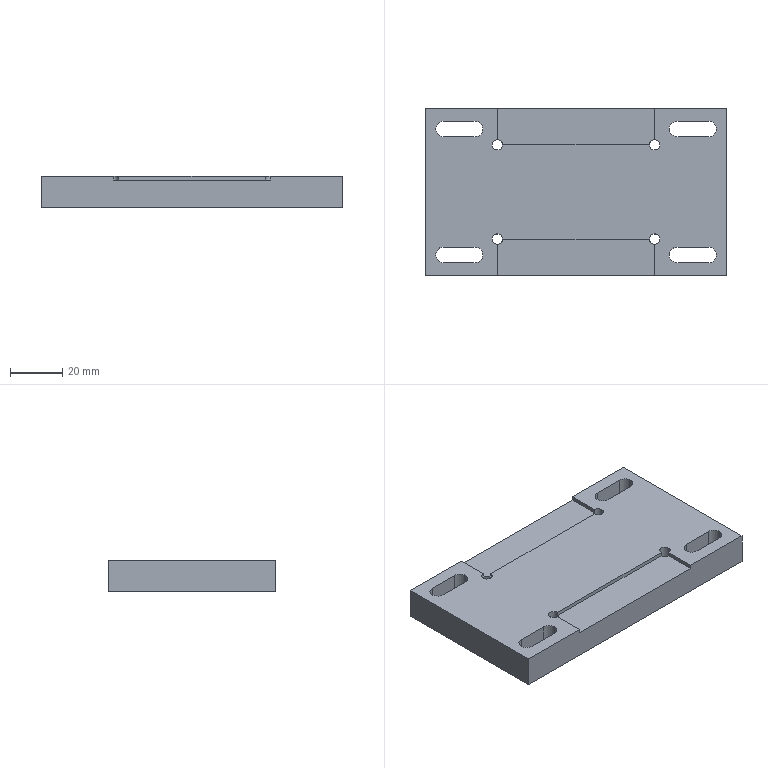Part | SolidWorks | features ICE 3, 3DProfileFeature 1, Extrusion 1, HoleWzd 1, MirrorPattern 1 | 1 solid | 46 faces | box 115 x 64 x 12 mm | volume 80039 mm3 | cylinder 22 | plane 22 | cone 2 | commonest cylinder face diameters 6 x12 4 x8 5 x2
STEP:
#1=CARTESIAN_POINT('',(39.5,0.,2.5));
#2=VERTEX_POINT('',#1);
#3=CARTESIAN_POINT('',(39.5,0.,-2.5));
#4=VERTEX_POINT('',#3);
#5=CARTESIAN_POINT('',(39.5,0.,0.));
#6=DIRECTION('',(1.,0.,0.));
#7=DIRECTION('',(0.,0.,-1.));
#8=AXIS2_PLACEMENT_3D('',#5,#6,#7);
#9=CIRCLE('',#8,2.5);
#10=EDGE_CURVE('',#2,#4,#9,.T.);
#11=ORIENTED_EDGE('',*,*,#10,.F.);
#12=CARTESIAN_POINT('',(57.5,0.,2.5));
#13=VERTEX_POINT('',#12);
#14=CARTESIAN_POINT('',(57.5,0.,2.5));
#15=DIRECTION('',(1.,0.,0.));
#16=VECTOR('',#15,1000.);
#17=LINE('',#14,#16);
#18=EDGE_CURVE('',#2,#13,#17,.T.);
#19=ORIENTED_EDGE('',*,*,#18,.T.);
#20=CARTESIAN_POINT('',(57.5,0.,-2.5));
#21=VERTEX_POINT('',#20);
#22=CARTESIAN_POINT('',(57.5,0.,0.));
#23=DIRECTION('',(1.,0.,0.));
#24=DIRECTION('',(0.,0.,-1.));
#25=AXIS2_PLACEMENT_3D('',#22,#23,#24);
#26=CIRCLE('',#25,2.5);
#27=EDGE_CURVE('',#13,#21,#26,.T.);
#28=ORIENTED_EDGE('',*,*,#27,.T.);
#29=CARTESIAN_POINT('',(57.5,0.,-2.5));
#30=DIRECTION('',(1.,0.,0.));
#31=VECTOR('',#30,1000.);
#32=LINE('',#29,#31);
#33=EDGE_CURVE('',#4,#21,#32,.T.);
#34=ORIENTED_EDGE('',*,*,#33,.F.);
#35=EDGE_LOOP('',(#11,#19,#28,#34));
#36=FACE_OUTER_BOUND('',#35,.T.);
#37=CARTESIAN_POINT('',(57.5,0.,0.));
#38=DIRECTION('',(1.,0.,0.));
#39=DIRECTION('',(0.,0.,-1.));
#40=AXIS2_PLACEMENT_3D('',#37,#38,#39);
#41=CYLINDRICAL_SURFACE('',#40,2.5);
#42=ADVANCED_FACE('',(#36),#41,.F.);
#43=CARTESIAN_POINT('',(37.998,0.,0.));
#44=VERTEX_POINT('',#43);
#45=CARTESIAN_POINT('',(39.5,0.,-2.5));
#46=DIRECTION('',(0.515,0.,-0.8572));
#47=VECTOR('',#46,1000.);
#48=LINE('',#45,#47);
#49=EDGE_CURVE('',#44,#4,#48,.T.);
#50=ORIENTED_EDGE('',*,*,#49,.F.);
#51=CARTESIAN_POINT('',(39.5,0.,2.5));
#52=DIRECTION('',(0.515,0.,0.8572));
#53=VECTOR('',#52,1000.);
#54=LINE('',#51,#53);
#55=EDGE_CURVE('',#44,#2,#54,.T.);
#56=ORIENTED_EDGE('',*,*,#55,.T.);
#57=ORIENTED_EDGE('',*,*,#10,.T.);
#58=EDGE_LOOP('',(#50,#56,#57));
#59=FACE_OUTER_BOUND('',#58,.T.);
#60=CARTESIAN_POINT('',(39.5,0.,0.));
#61=DIRECTION('',(1.,0.,0.));
#62=DIRECTION('',(0.,0.,-1.));
#63=AXIS2_PLACEMENT_3D('',#60,#61,#62);
#64=CONICAL_SURFACE('',#63,2.5,1.03);
#65=ADVANCED_FACE('',(#59),#64,.F.);
#66=CARTESIAN_POINT('',(53.5,24.,-6.));
#67=VERTEX_POINT('',#66);
#68=CARTESIAN_POINT('',(50.5,27.,-6.));
#69=VERTEX_POINT('',#68);
#70=CARTESIAN_POINT('',(50.5,24.,-6.));
#71=DIRECTION('',(0.,0.,1.));
#72=DIRECTION('',(-1.,0.,0.));
#73=AXIS2_PLACEMENT_3D('',#70,#71,#72);
#74=CIRCLE('',#73,3.);
#75=EDGE_CURVE('',#67,#69,#74,.T.);
#76=ORIENTED_EDGE('',*,*,#75,.F.);
#77=CARTESIAN_POINT('',(53.5,24.,6.));
#78=VERTEX_POINT('',#77);
#79=CARTESIAN_POINT('',(53.5,24.,-6.001));
#80=DIRECTION('',(0.,0.,1.));
#81=VECTOR('',#80,1000.);
#82=LINE('',#79,#81);
#83=EDGE_CURVE('',#67,#78,#82,.T.);
#84=ORIENTED_EDGE('',*,*,#83,.T.);
#85=CARTESIAN_POINT('',(50.5,27.,6.));
#86=VERTEX_POINT('',#85);
#87=CARTESIAN_POINT('',(50.5,24.,6.));
#88=DIRECTION('',(0.,0.,1.));
#89=DIRECTION('',(-1.,0.,0.));
#90=AXIS2_PLACEMENT_3D('',#87,#88,#89);
#91=CIRCLE('',#90,3.);
#92=EDGE_CURVE('',#78,#86,#91,.T.);
#93=ORIENTED_EDGE('',*,*,#92,.T.);
#94=CARTESIAN_POINT('',(50.5,27.,-6.001));
#95=DIRECTION('',(0.,0.,1.));
#96=VECTOR('',#95,1000.);
#97=LINE('',#94,#96);
#98=EDGE_CURVE('',#69,#86,#97,.T.);
#99=ORIENTED_EDGE('',*,*,#98,.F.);
#100=EDGE_LOOP('',(#76,#84,#93,#99));
#101=FACE_OUTER_BOUND('',#100,.T.);
#102=CARTESIAN_POINT('',(50.5,24.,-6.001));
#103=DIRECTION('',(0.,0.,1.));
#104=DIRECTION('',(1.,0.,0.));
#105=AXIS2_PLACEMENT_3D('',#102,#103,#104);
#106=CYLINDRICAL_SURFACE('',#105,3.);
#107=ADVANCED_FACE('',(#101),#106,.F.);
#108=CARTESIAN_POINT('',(-35.5,-24.,-6.));
#109=VERTEX_POINT('',#108);
#110=CARTESIAN_POINT('',(-38.5,-21.,-6.));
#111=VERTEX_POINT('',#110);
#112=CARTESIAN_POINT('',(-38.5,-24.,-6.));
#113=DIRECTION('',(0.,0.,1.));
#114=DIRECTION('',(-1.,0.,0.));
#115=AXIS2_PLACEMENT_3D('',#112,#113,#114);
#116=CIRCLE('',#115,3.);
#117=EDGE_CURVE('',#109,#111,#116,.T.);
#118=ORIENTED_EDGE('',*,*,#117,.F.);
#119=CARTESIAN_POINT('',(-35.5,-24.,6.));
#120=VERTEX_POINT('',#119);
#121=CARTESIAN_POINT('',(-35.5,-24.,-6.001));
#122=DIRECTION('',(0.,0.,1.));
#123=VECTOR('',#122,1000.);
#124=LINE('',#121,#123);
#125=EDGE_CURVE('',#109,#120,#124,.T.);
#126=ORIENTED_EDGE('',*,*,#125,.T.);
#127=CARTESIAN_POINT('',(-38.5,-21.,6.));
#128=VERTEX_POINT('',#127);
#129=CARTESIAN_POINT('',(-38.5,-24.,6.));
#130=DIRECTION('',(0.,0.,1.));
#131=DIRECTION('',(-1.,0.,0.));
#132=AXIS2_PLACEMENT_3D('',#129,#130,#131);
#133=CIRCLE('',#132,3.);
#134=EDGE_CURVE('',#120,#128,#133,.T.);
#135=ORIENTED_EDGE('',*,*,#134,.T.);
#136=CARTESIAN_POINT('',(-38.5,-21.,-6.001));
#137=DIRECTION('',(0.,0.,1.));
#138=VECTOR('',#137,1000.);
#139=LINE('',#136,#138);
#140=EDGE_CURVE('',#111,#128,#139,.T.);
#141=ORIENTED_EDGE('',*,*,#140,.F.);
#142=EDGE_LOOP('',(#118,#126,#135,#141));
#143=FACE_OUTER_BOUND('',#142,.T.);
#144=CARTESIAN_POINT('',(-38.5,-24.,-6.001));
#145=DIRECTION('',(0.,0.,1.));
#146=DIRECTION('',(1.,0.,0.));
#147=AXIS2_PLACEMENT_3D('',#144,#145,#146);
#148=CYLINDRICAL_SURFACE('',#147,3.);
#149=ADVANCED_FACE('',(#143),#148,.F.);
#150=CARTESIAN_POINT('',(53.5,-24.,-6.));
#151=VERTEX_POINT('',#150);
#152=CARTESIAN_POINT('',(50.5,-21.,-6.));
#153=VERTEX_POINT('',#152);
#154=CARTESIAN_POINT('',(50.5,-24.,-6.));
#155=DIRECTION('',(0.,0.,1.));
#156=DIRECTION('',(-1.,0.,0.));
#157=AXIS2_PLACEMENT_3D('',#154,#155,#156);
#158=CIRCLE('',#157,3.);
#159=EDGE_CURVE('',#151,#153,#158,.T.);
#160=ORIENTED_EDGE('',*,*,#159,.F.);
#161=CARTESIAN_POINT('',(53.5,-24.,6.));
#162=VERTEX_POINT('',#161);
#163=CARTESIAN_POINT('',(53.5,-24.,-6.001));
#164=DIRECTION('',(0.,0.,1.));
#165=VECTOR('',#164,1000.);
#166=LINE('',#163,#165);
#167=EDGE_CURVE('',#151,#162,#166,.T.);
#168=ORIENTED_EDGE('',*,*,#167,.T.);
#169=CARTESIAN_POINT('',(50.5,-21.,6.));
#170=VERTEX_POINT('',#169);
#171=CARTESIAN_POINT('',(50.5,-24.,6.));
#172=DIRECTION('',(0.,0.,1.));
#173=DIRECTION('',(1.,0.,0.));
#174=AXIS2_PLACEMENT_3D('',#171,#172,#173);
#175=CIRCLE('',#174,3.);
#176=EDGE_CURVE('',#162,#170,#175,.T.);
#177=ORIENTED_EDGE('',*,*,#176,.T.);
#178=CARTESIAN_POINT('',(50.5,-21.,-6.001));
#179=DIRECTION('',(0.,0.,1.));
#180=VECTOR('',#179,1000.);
#181=LINE('',#178,#180);
#182=EDGE_CURVE('',#153,#170,#181,.T.);
#183=ORIENTED_EDGE('',*,*,#182,.F.);
#184=EDGE_LOOP('',(#160,#168,#177,#183));
#185=FACE_OUTER_BOUND('',#184,.T.);
#186=CARTESIAN_POINT('',(50.5,-24.,-6.001));
#187=DIRECTION('',(0.,0.,1.));
#188=DIRECTION('',(1.,0.,0.));
#189=AXIS2_PLACEMENT_3D('',#186,#187,#188);
#190=CYLINDRICAL_SURFACE('',#189,3.);
#191=ADVANCED_FACE('',(#185),#190,.F.);
#192=CARTESIAN_POINT('',(-35.5,24.,-6.));
#193=VERTEX_POINT('',#192);
#194=CARTESIAN_POINT('',(-38.5,27.,-6.));
#195=VERTEX_POINT('',#194);
#196=CARTESIAN_POINT('',(-38.5,24.,-6.));
#197=DIRECTION('',(0.,0.,1.));
#198=DIRECTION('',(-1.,0.,0.));
#199=AXIS2_PLACEMENT_3D('',#196,#197,#198);
#200=CIRCLE('',#199,3.);
#201=EDGE_CURVE('',#193,#195,#200,.T.);
#202=ORIENTED_EDGE('',*,*,#201,.F.);
#203=CARTESIAN_POINT('',(-35.5,24.,6.));
#204=VERTEX_POINT('',#203);
#205=CARTESIAN_POINT('',(-35.5,24.,-6.001));
#206=DIRECTION('',(0.,0.,1.));
#207=VECTOR('',#206,1000.);
#208=LINE('',#205,#207);
#209=EDGE_CURVE('',#193,#204,#208,.T.);
#210=ORIENTED_EDGE('',*,*,#209,.T.);
#211=CARTESIAN_POINT('',(-38.5,27.,6.));
#212=VERTEX_POINT('',#211);
#213=CARTESIAN_POINT('',(-38.5,24.,6.));
#214=DIRECTION('',(0.,0.,1.));
#215=DIRECTION('',(1.,0.,0.));
#216=AXIS2_PLACEMENT_3D('',#213,#214,#215);
#217=CIRCLE('',#216,3.);
#218=EDGE_CURVE('',#204,#212,#217,.T.);
#219=ORIENTED_EDGE('',*,*,#218,.T.);
#220=CARTESIAN_POINT('',(-38.5,27.,-6.001));
#221=DIRECTION('',(0.,0.,1.));
#222=VECTOR('',#221,1000.);
#223=LINE('',#220,#222);
#224=EDGE_CURVE('',#195,#212,#223,.T.);
#225=ORIENTED_EDGE('',*,*,#224,.F.);
#226=EDGE_LOOP('',(#202,#210,#219,#225));
#227=FACE_OUTER_BOUND('',#226,.T.);
#228=CARTESIAN_POINT('',(-38.5,24.,-6.001));
#229=DIRECTION('',(0.,0.,1.));
#230=DIRECTION('',(1.,0.,0.));
#231=AXIS2_PLACEMENT_3D('',#228,#229,#230);
#232=CYLINDRICAL_SURFACE('',#231,3.);
#233=ADVANCED_FACE('',(#227),#232,.F.);
#234=CARTESIAN_POINT('',(-28.,-18.,-6.));
#235=VERTEX_POINT('',#234);
#236=CARTESIAN_POINT('',(-32.,-18.,-6.));
#237=VERTEX_POINT('',#236);
#238=CARTESIAN_POINT('',(-30.,-18.,-6.));
#239=DIRECTION('',(0.,0.,-1.));
#240=DIRECTION('',(1.,0.,0.));
#241=AXIS2_PLACEMENT_3D('',#238,#239,#240);
#242=CIRCLE('',#241,2.);
#243=EDGE_CURVE('',#235,#237,#242,.T.);
#244=ORIENTED_EDGE('',*,*,#243,.T.);
#245=CARTESIAN_POINT('',(-32.,-18.,6.));
#246=VERTEX_POINT('',#245);
#247=CARTESIAN_POINT('',(-32.,-18.,-6.));
#248=DIRECTION('',(0.,0.,1.));
#249=VECTOR('',#248,1000.);
#250=LINE('',#247,#249);
#251=EDGE_CURVE('',#237,#246,#250,.T.);
#252=ORIENTED_EDGE('',*,*,#251,.T.);
#253=CARTESIAN_POINT('',(-30.,-20.,6.));
#254=VERTEX_POINT('',#253);
#255=CARTESIAN_POINT('',(-30.,-18.,6.));
#256=DIRECTION('',(0.,0.,1.));
#257=DIRECTION('',(-1.,0.,0.));
#258=AXIS2_PLACEMENT_3D('',#255,#256,#257);
#259=CIRCLE('',#258,2.);
#260=EDGE_CURVE('',#246,#254,#259,.T.);
#261=ORIENTED_EDGE('',*,*,#260,.T.);
#262=CARTESIAN_POINT('',(-30.,-20.,4.5));
#263=VERTEX_POINT('',#262);
#264=CARTESIAN_POINT('',(-30.,-20.,-6.));
#265=DIRECTION('',(0.,0.,1.));
#266=VECTOR('',#265,1000.);
#267=LINE('',#264,#266);
#268=EDGE_CURVE('',#263,#254,#267,.T.);
#269=ORIENTED_EDGE('',*,*,#268,.F.);
#270=CARTESIAN_POINT('',(-28.,-18.,4.5));
#271=VERTEX_POINT('',#270);
#272=CARTESIAN_POINT('',(-30.,-18.,4.5));
#273=DIRECTION('',(0.,0.,1.));
#274=DIRECTION('',(-1.,0.,0.));
#275=AXIS2_PLACEMENT_3D('',#272,#273,#274);
#276=CIRCLE('',#275,2.);
#277=EDGE_CURVE('',#263,#271,#276,.T.);
#278=ORIENTED_EDGE('',*,*,#277,.T.);
#279=CARTESIAN_POINT('',(-28.,-18.,-6.));
#280=DIRECTION('',(0.,0.,1.));
#281=VECTOR('',#280,1000.);
#282=LINE('',#279,#281);
#283=EDGE_CURVE('',#235,#271,#282,.T.);
#284=ORIENTED_EDGE('',*,*,#283,.F.);
#285=EDGE_LOOP('',(#244,#252,#261,#269,#278,#284));
#286=FACE_OUTER_BOUND('',#285,.T.);
#287=CARTESIAN_POINT('',(-30.,-18.,-6.));
#288=DIRECTION('',(0.,0.,1.));
#289=DIRECTION('',(1.,0.,0.));
#290=AXIS2_PLACEMENT_3D('',#287,#288,#289);
#291=CYLINDRICAL_SURFACE('',#290,2.);
#292=ADVANCED_FACE('',(#286),#291,.F.);
#293=CARTESIAN_POINT('',(32.,-18.,-6.));
#294=VERTEX_POINT('',#293);
#295=CARTESIAN_POINT('',(28.,-18.,-6.));
#296=VERTEX_POINT('',#295);
#297=CARTESIAN_POINT('',(30.,-18.,-6.));
#298=DIRECTION('',(0.,0.,-1.));
#299=DIRECTION('',(1.,0.,0.));
#300=AXIS2_PLACEMENT_3D('',#297,#298,#299);
#301=CIRCLE('',#300,2.);
#302=EDGE_CURVE('',#294,#296,#301,.T.);
#303=ORIENTED_EDGE('',*,*,#302,.T.);
#304=CARTESIAN_POINT('',(28.,-18.,4.5));
#305=VERTEX_POINT('',#304);
#306=CARTESIAN_POINT('',(28.,-18.,-6.));
#307=DIRECTION('',(0.,0.,1.));
#308=VECTOR('',#307,1000.);
#309=LINE('',#306,#308);
#310=EDGE_CURVE('',#296,#305,#309,.T.);
#311=ORIENTED_EDGE('',*,*,#310,.T.);
#312=CARTESIAN_POINT('',(30.,-20.,4.5));
#313=VERTEX_POINT('',#312);
#314=CARTESIAN_POINT('',(30.,-18.,4.5));
#315=DIRECTION('',(0.,0.,1.));
#316=DIRECTION('',(-1.,0.,0.));
#317=AXIS2_PLACEMENT_3D('',#314,#315,#316);
#318=CIRCLE('',#317,2.);
#319=EDGE_CURVE('',#305,#313,#318,.T.);
#320=ORIENTED_EDGE('',*,*,#319,.T.);
#321=CARTESIAN_POINT('',(30.,-20.,6.));
#322=VERTEX_POINT('',#321);
#323=CARTESIAN_POINT('',(30.,-20.,-6.));
#324=DIRECTION('',(0.,0.,-1.));
#325=VECTOR('',#324,1000.);
#326=LINE('',#323,#325);
#327=EDGE_CURVE('',#322,#313,#326,.T.);
#328=ORIENTED_EDGE('',*,*,#327,.F.);
#329=CARTESIAN_POINT('',(32.,-18.,6.));
#330=VERTEX_POINT('',#329);
#331=CARTESIAN_POINT('',(30.,-18.,6.));
#332=DIRECTION('',(0.,0.,1.));
#333=DIRECTION('',(-1.,0.,0.));
#334=AXIS2_PLACEMENT_3D('',#331,#332,#333);
#335=CIRCLE('',#334,2.);
#336=EDGE_CURVE('',#322,#330,#335,.T.);
#337=ORIENTED_EDGE('',*,*,#336,.T.);
#338=CARTESIAN_POINT('',(32.,-18.,-6.));
#339=DIRECTION('',(0.,0.,1.));
#340=VECTOR('',#339,1000.);
#341=LINE('',#338,#340);
#342=EDGE_CURVE('',#294,#330,#341,.T.);
#343=ORIENTED_EDGE('',*,*,#342,.F.);
#344=EDGE_LOOP('',(#303,#311,#320,#328,#337,#343));
#345=FACE_OUTER_BOUND('',#344,.T.);
#346=CARTESIAN_POINT('',(30.,-18.,-6.));
#347=DIRECTION('',(0.,0.,1.));
#348=DIRECTION('',(1.,0.,0.));
#349=AXIS2_PLACEMENT_3D('',#346,#347,#348);
#350=CYLINDRICAL_SURFACE('',#349,2.);
#351=ADVANCED_FACE('',(#345),#350,.F.);
#352=CARTESIAN_POINT('',(-32.,18.,-6.));
#353=VERTEX_POINT('',#352);
#354=CARTESIAN_POINT('',(-28.,18.,-6.));
#355=VERTEX_POINT('',#354);
#356=CARTESIAN_POINT('',(-30.,18.,-6.));
#357=DIRECTION('',(0.,0.,1.));
#358=DIRECTION('',(1.,0.,0.));
#359=AXIS2_PLACEMENT_3D('',#356,#357,#358);
#360=CIRCLE('',#359,2.);
#361=EDGE_CURVE('',#353,#355,#360,.T.);
#362=ORIENTED_EDGE('',*,*,#361,.F.);
#363=CARTESIAN_POINT('',(-32.,18.,6.));
#364=VERTEX_POINT('',#363);
#365=CARTESIAN_POINT('',(-32.,18.,-6.));
#366=DIRECTION('',(0.,0.,1.));
#367=VECTOR('',#366,1000.);
#368=LINE('',#365,#367);
#369=EDGE_CURVE('',#353,#364,#368,.T.);
#370=ORIENTED_EDGE('',*,*,#369,.T.);
#371=CARTESIAN_POINT('',(-28.,18.,6.));
#372=VERTEX_POINT('',#371);
#373=CARTESIAN_POINT('',(-30.,18.,6.));
#374=DIRECTION('',(0.,0.,-1.));
#375=DIRECTION('',(-1.,0.,0.));
#376=AXIS2_PLACEMENT_3D('',#373,#374,#375);
#377=CIRCLE('',#376,2.);
#378=EDGE_CURVE('',#372,#364,#377,.T.);
#379=ORIENTED_EDGE('',*,*,#378,.F.);
#380=CARTESIAN_POINT('',(-28.,18.,4.5));
#381=VERTEX_POINT('',#380);
#382=CARTESIAN_POINT('',(-28.,18.,-6.));
#383=DIRECTION('',(0.,0.,1.));
#384=VECTOR('',#383,1000.);
#385=LINE('',#382,#384);
#386=EDGE_CURVE('',#381,#372,#385,.T.);
#387=ORIENTED_EDGE('',*,*,#386,.F.);
#388=CARTESIAN_POINT('',(-28.,18.,-6.));
#389=DIRECTION('',(0.,0.,1.));
#390=VECTOR('',#389,1000.);
#391=LINE('',#388,#390);
#392=EDGE_CURVE('',#355,#381,#391,.T.);
#393=ORIENTED_EDGE('',*,*,#392,.F.);
#394=EDGE_LOOP('',(#362,#370,#379,#387,#393));
#395=FACE_OUTER_BOUND('',#394,.T.);
#396=CARTESIAN_POINT('',(-30.,18.,-6.));
#397=DIRECTION('',(0.,0.,1.));
#398=DIRECTION('',(1.,0.,0.));
#399=AXIS2_PLACEMENT_3D('',#396,#397,#398);
#400=CYLINDRICAL_SURFACE('',#399,2.);
#401=ADVANCED_FACE('',(#395),#400,.F.);
#402=CARTESIAN_POINT('',(28.,18.,-6.));
#403=VERTEX_POINT('',#402);
#404=CARTESIAN_POINT('',(32.,18.,-6.));
#405=VERTEX_POINT('',#404);
#406=CARTESIAN_POINT('',(30.,18.,-6.));
#407=DIRECTION('',(0.,0.,1.));
#408=DIRECTION('',(1.,0.,0.));
#409=AXIS2_PLACEMENT_3D('',#406,#407,#408);
#410=CIRCLE('',#409,2.);
#411=EDGE_CURVE('',#403,#405,#410,.T.);
#412=ORIENTED_EDGE('',*,*,#411,.F.);
#413=CARTESIAN_POINT('',(28.,18.,4.5));
#414=VERTEX_POINT('',#413);
#415=CARTESIAN_POINT('',(28.,18.,-6.));
#416=DIRECTION('',(0.,0.,1.));
#417=VECTOR('',#416,1000.);
#418=LINE('',#415,#417);
#419=EDGE_CURVE('',#403,#414,#418,.T.);
#420=ORIENTED_EDGE('',*,*,#419,.T.);
#421=CARTESIAN_POINT('',(28.,18.,6.));
#422=VERTEX_POINT('',#421);
#423=CARTESIAN_POINT('',(28.,18.,-6.));
#424=DIRECTION('',(0.,0.,-1.));
#425=VECTOR('',#424,1000.);
#426=LINE('',#423,#425);
#427=EDGE_CURVE('',#422,#414,#426,.T.);
#428=ORIENTED_EDGE('',*,*,#427,.F.);
#429=CARTESIAN_POINT('',(32.,18.,6.));
#430=VERTEX_POINT('',#429);
#431=CARTESIAN_POINT('',(30.,18.,6.));
#432=DIRECTION('',(0.,0.,-1.));
#433=DIRECTION('',(-1.,0.,0.));
#434=AXIS2_PLACEMENT_3D('',#431,#432,#433);
#435=CIRCLE('',#434,2.);
#436=EDGE_CURVE('',#430,#422,#435,.T.);
#437=ORIENTED_EDGE('',*,*,#436,.F.);
#438=CARTESIAN_POINT('',(32.,18.,-6.));
#439=DIRECTION('',(0.,0.,1.));
#440=VECTOR('',#439,1000.);
#441=LINE('',#438,#440);
#442=EDGE_CURVE('',#405,#430,#441,.T.);
#443=ORIENTED_EDGE('',*,*,#442,.F.);
#444=EDGE_LOOP('',(#412,#420,#428,#437,#443));
#445=FACE_OUTER_BOUND('',#444,.T.);
#446=CARTESIAN_POINT('',(30.,18.,-6.));
#447=DIRECTION('',(0.,0.,1.));
#448=DIRECTION('',(1.,0.,0.));
#449=AXIS2_PLACEMENT_3D('',#446,#447,#448);
#450=CYLINDRICAL_SURFACE('',#449,2.);
#451=ADVANCED_FACE('',(#445),#450,.F.);
#452=CARTESIAN_POINT('',(30.,-32.,6.));
#453=VERTEX_POINT('',#452);
#454=CARTESIAN_POINT('',(30.,-18.,6.));
#455=DIRECTION('',(0.,-1.,0.));
#456=VECTOR('',#455,1000.);
#457=LINE('',#454,#456);
#458=EDGE_CURVE('',#322,#453,#457,.T.);
#459=ORIENTED_EDGE('',*,*,#458,.F.);
#460=ORIENTED_EDGE('',*,*,#327,.T.);
#461=CARTESIAN_POINT('',(30.,-32.,4.5));
#462=VERTEX_POINT('',#461);
#463=CARTESIAN_POINT('',(30.,-18.,4.5));
#464=DIRECTION('',(0.,-1.,0.));
#465=VECTOR('',#464,1000.);
#466=LINE('',#463,#465);
#467=EDGE_CURVE('',#313,#462,#466,.T.);
#468=ORIENTED_EDGE('',*,*,#467,.T.);
#469=CARTESIAN_POINT('',(30.,-32.,4.5));
#470=DIRECTION('',(0.,0.,1.));
#471=VECTOR('',#470,1000.);
#472=LINE('',#469,#471);
#473=EDGE_CURVE('',#462,#453,#472,.T.);
#474=ORIENTED_EDGE('',*,*,#473,.T.);
#475=EDGE_LOOP('',(#459,#460,#468,#474));
#476=FACE_OUTER_BOUND('',#475,.T.);
#477=CARTESIAN_POINT('',(30.,-18.,4.5));
#478=DIRECTION('',(-1.,0.,0.));
#479=DIRECTION('',(0.,0.,1.));
#480=AXIS2_PLACEMENT_3D('',#477,#478,#479);
#481=PLANE('',#480);
#482=ADVANCED_FACE('',(#476),#481,.T.);
#483=CARTESIAN_POINT('',(-30.,-32.,4.5));
#484=VERTEX_POINT('',#483);
#485=CARTESIAN_POINT('',(-30.,-18.,4.5));
#486=DIRECTION('',(0.,1.,0.));
#487=VECTOR('',#486,1000.);
#488=LINE('',#485,#487);
#489=EDGE_CURVE('',#484,#263,#488,.T.);
#490=ORIENTED_EDGE('',*,*,#489,.T.);
#491=ORIENTED_EDGE('',*,*,#268,.T.);
#492=CARTESIAN_POINT('',(-30.,-32.,6.));
#493=VERTEX_POINT('',#492);
#494=CARTESIAN_POINT('',(-30.,-18.,6.));
#495=DIRECTION('',(0.,1.,0.));
#496=VECTOR('',#495,1000.);
#497=LINE('',#494,#496);
#498=EDGE_CURVE('',#493,#254,#497,.T.);
#499=ORIENTED_EDGE('',*,*,#498,.F.);
#500=CARTESIAN_POINT('',(-30.,-32.,4.5));
#501=DIRECTION('',(0.,0.,1.));
#502=VECTOR('',#501,1000.);
#503=LINE('',#500,#502);
#504=EDGE_CURVE('',#484,#493,#503,.T.);
#505=ORIENTED_EDGE('',*,*,#504,.F.);
#506=EDGE_LOOP('',(#490,#491,#499,#505));
#507=FACE_OUTER_BOUND('',#506,.T.);
#508=CARTESIAN_POINT('',(-30.,-18.,4.5));
#509=DIRECTION('',(1.,0.,0.));
#510=DIRECTION('',(0.,0.,-1.));
#511=AXIS2_PLACEMENT_3D('',#508,#509,#510);
#512=PLANE('',#511);
#513=ADVANCED_FACE('',(#507),#512,.T.);
#514=CARTESIAN_POINT('',(-28.,-18.,6.));
#515=VERTEX_POINT('',#514);
#516=CARTESIAN_POINT('',(28.,-18.,6.));
#517=VERTEX_POINT('',#516);
#518=CARTESIAN_POINT('',(-30.,-18.,6.));
#519=DIRECTION('',(1.,0.,0.));
#520=VECTOR('',#519,1000.);
#521=LINE('',#518,#520);
#522=EDGE_CURVE('',#515,#517,#521,.T.);
#523=ORIENTED_EDGE('',*,*,#522,.F.);
#524=CARTESIAN_POINT('',(-28.,-18.,-6.));
#525=DIRECTION('',(0.,0.,-1.));
#526=VECTOR('',#525,1000.);
#527=LINE('',#524,#526);
#528=EDGE_CURVE('',#515,#271,#527,.T.);
#529=ORIENTED_EDGE('',*,*,#528,.T.);
#530=CARTESIAN_POINT('',(-30.,-18.,4.5));
#531=DIRECTION('',(1.,0.,0.));
#532=VECTOR('',#531,1000.);
#533=LINE('',#530,#532);
#534=EDGE_CURVE('',#271,#305,#533,.T.);
#535=ORIENTED_EDGE('',*,*,#534,.T.);
#536=CARTESIAN_POINT('',(28.,-18.,-6.));
#537=DIRECTION('',(0.,0.,1.));
#538=VECTOR('',#537,1000.);
#539=LINE('',#536,#538);
#540=EDGE_CURVE('',#305,#517,#539,.T.);
#541=ORIENTED_EDGE('',*,*,#540,.T.);
#542=EDGE_LOOP('',(#523,#529,#535,#541));
#543=FACE_OUTER_BOUND('',#542,.T.);
#544=CARTESIAN_POINT('',(-30.,-18.,4.5));
#545=DIRECTION('',(0.,-1.,0.));
#546=DIRECTION('',(0.,0.,-1.));
#547=AXIS2_PLACEMENT_3D('',#544,#545,#546);
#548=PLANE('',#547);
#549=ADVANCED_FACE('',(#543),#548,.T.);
#550=ORIENTED_EDGE('',*,*,#473,.F.);
#551=CARTESIAN_POINT('',(-30.,-32.,4.5));
#552=DIRECTION('',(-1.,0.,0.));
#553=VECTOR('',#552,1000.);
#554=LINE('',#551,#553);
#555=EDGE_CURVE('',#462,#484,#554,.T.);
#556=ORIENTED_EDGE('',*,*,#555,.T.);
#557=ORIENTED_EDGE('',*,*,#504,.T.);
#558=CARTESIAN_POINT('',(-57.5,-32.,6.));
#559=VERTEX_POINT('',#558);
#560=CARTESIAN_POINT('',(-57.5,-32.,6.));
#561=DIRECTION('',(1.,0.,0.));
#562=VECTOR('',#561,1000.);
#563=LINE('',#560,#562);
#564=EDGE_CURVE('',#559,#493,#563,.T.);
#565=ORIENTED_EDGE('',*,*,#564,.F.);
#566=CARTESIAN_POINT('',(-57.5,-32.,-6.));
#567=VERTEX_POINT('',#566);
#568=CARTESIAN_POINT('',(-57.5,-32.,6.));
#569=DIRECTION('',(0.,0.,-1.));
#570=VECTOR('',#569,1000.);
#571=LINE('',#568,#570);
#572=EDGE_CURVE('',#559,#567,#571,.T.);
#573=ORIENTED_EDGE('',*,*,#572,.T.);
#574=CARTESIAN_POINT('',(57.5,-32.,-6.));
#575=VERTEX_POINT('',#574);
#576=CARTESIAN_POINT('',(-57.5,-32.,-6.));
#577=DIRECTION('',(1.,0.,0.));
#578=VECTOR('',#577,1000.);
#579=LINE('',#576,#578);
#580=EDGE_CURVE('',#567,#575,#579,.T.);
#581=ORIENTED_EDGE('',*,*,#580,.T.);
#582=CARTESIAN_POINT('',(57.5,-32.,6.));
#583=VERTEX_POINT('',#582);
#584=CARTESIAN_POINT('',(57.5,-32.,6.));
#585=DIRECTION('',(0.,0.,-1.));
#586=VECTOR('',#585,1000.);
#587=LINE('',#584,#586);
#588=EDGE_CURVE('',#583,#575,#587,.T.);
#589=ORIENTED_EDGE('',*,*,#588,.F.);
#590=CARTESIAN_POINT('',(-57.5,-32.,6.));
#591=DIRECTION('',(1.,0.,0.));
#592=VECTOR('',#591,1000.);
#593=LINE('',#590,#592);
#594=EDGE_CURVE('',#453,#583,#593,.T.);
#595=ORIENTED_EDGE('',*,*,#594,.F.);
#596=EDGE_LOOP('',(#550,#556,#557,#565,#573,#581,#589,#595));
#597=FACE_OUTER_BOUND('',#596,.T.);
#598=CARTESIAN_POINT('',(-57.5,-32.,6.));
#599=DIRECTION('',(0.,1.,0.));
#600=DIRECTION('',(0.,0.,1.));
#601=AXIS2_PLACEMENT_3D('',#598,#599,#600);
#602=PLANE('',#601);
#603=ADVANCED_FACE('',(#597),#602,.F.);
#604=CARTESIAN_POINT('',(38.5,27.,6.));
#605=VERTEX_POINT('',#604);
#606=CARTESIAN_POINT('',(50.5,27.,6.));
#607=DIRECTION('',(-1.,0.,0.));
#608=VECTOR('',#607,1000.);
#609=LINE('',#606,#608);
#610=EDGE_CURVE('',#86,#605,#609,.T.);
#611=ORIENTED_EDGE('',*,*,#610,.F.);
#612=ORIENTED_EDGE('',*,*,#92,.F.);
#613=CARTESIAN_POINT('',(50.5,21.,6.));
#614=VERTEX_POINT('',#613);
#615=CARTESIAN_POINT('',(50.5,24.,6.));
#616=DIRECTION('',(0.,0.,1.));
#617=DIRECTION('',(-1.,0.,0.));
#618=AXIS2_PLACEMENT_3D('',#615,#616,#617);
#619=CIRCLE('',#618,3.);
#620=EDGE_CURVE('',#614,#78,#619,.T.);
#621=ORIENTED_EDGE('',*,*,#620,.F.);
#622=CARTESIAN_POINT('',(38.5,21.,6.));
#623=VERTEX_POINT('',#622);
#624=CARTESIAN_POINT('',(50.5,21.,6.));
#625=DIRECTION('',(1.,0.,0.));
#626=VECTOR('',#625,1000.);
#627=LINE('',#624,#626);
#628=EDGE_CURVE('',#623,#614,#627,.T.);
#629=ORIENTED_EDGE('',*,*,#628,.F.);
#630=CARTESIAN_POINT('',(38.5,24.,6.));
#631=DIRECTION('',(0.,0.,1.));
#632=DIRECTION('',(-1.,0.,0.));
#633=AXIS2_PLACEMENT_3D('',#630,#631,#632);
#634=CIRCLE('',#633,3.);
#635=EDGE_CURVE('',#605,#623,#634,.T.);
#636=ORIENTED_EDGE('',*,*,#635,.F.);
#637=EDGE_LOOP('',(#611,#612,#621,#629,#636));
#638=FACE_BOUND('',#637,.T.);
#639=CARTESIAN_POINT('',(-50.5,-27.,6.));
#640=VERTEX_POINT('',#639);
#641=CARTESIAN_POINT('',(-38.5,-27.,6.));
#642=VERTEX_POINT('',#641);
#643=CARTESIAN_POINT('',(-50.5,-27.,6.));
#644=DIRECTION('',(1.,0.,0.));
#645=VECTOR('',#644,1000.);
#646=LINE('',#643,#645);
#647=EDGE_CURVE('',#640,#642,#646,.T.);
#648=ORIENTED_EDGE('',*,*,#647,.F.);
#649=CARTESIAN_POINT('',(-50.5,-21.,6.));
#650=VERTEX_POINT('',#649);
#651=CARTESIAN_POINT('',(-50.5,-24.,6.));
#652=DIRECTION('',(0.,0.,1.));
#653=DIRECTION('',(-1.,0.,0.));
#654=AXIS2_PLACEMENT_3D('',#651,#652,#653);
#655=CIRCLE('',#654,3.);
#656=EDGE_CURVE('',#650,#640,#655,.T.);
#657=ORIENTED_EDGE('',*,*,#656,.F.);
#658=CARTESIAN_POINT('',(-50.5,-21.,6.));
#659=DIRECTION('',(-1.,0.,0.));
#660=VECTOR('',#659,1000.);
#661=LINE('',#658,#660);
#662=EDGE_CURVE('',#128,#650,#661,.T.);
#663=ORIENTED_EDGE('',*,*,#662,.F.);
#664=ORIENTED_EDGE('',*,*,#134,.F.);
#665=CARTESIAN_POINT('',(-38.5,-24.,6.));
#666=DIRECTION('',(0.,0.,1.));
#667=DIRECTION('',(-1.,0.,0.));
#668=AXIS2_PLACEMENT_3D('',#665,#666,#667);
#669=CIRCLE('',#668,3.);
#670=EDGE_CURVE('',#642,#120,#669,.T.);
#671=ORIENTED_EDGE('',*,*,#670,.F.);
#672=EDGE_LOOP('',(#648,#657,#663,#664,#671));
#673=FACE_BOUND('',#672,.T.);
#674=CARTESIAN_POINT('',(38.5,-21.,6.));
#675=VERTEX_POINT('',#674);
#676=CARTESIAN_POINT('',(50.5,-21.,6.));
#677=DIRECTION('',(-1.,0.,0.));
#678=VECTOR('',#677,1000.);
#679=LINE('',#676,#678);
#680=EDGE_CURVE('',#170,#675,#679,.T.);
#681=ORIENTED_EDGE('',*,*,#680,.F.);
#682=ORIENTED_EDGE('',*,*,#176,.F.);
#683=CARTESIAN_POINT('',(50.5,-27.,6.));
#684=VERTEX_POINT('',#683);
#685=CARTESIAN_POINT('',(50.5,-24.,6.));
#686=DIRECTION('',(0.,0.,1.));
#687=DIRECTION('',(1.,0.,0.));
#688=AXIS2_PLACEMENT_3D('',#685,#686,#687);
#689=CIRCLE('',#688,3.);
#690=EDGE_CURVE('',#684,#162,#689,.T.);
#691=ORIENTED_EDGE('',*,*,#690,.F.);
#692=CARTESIAN_POINT('',(38.5,-27.,6.));
#693=VERTEX_POINT('',#692);
#694=CARTESIAN_POINT('',(50.5,-27.,6.));
#695=DIRECTION('',(1.,0.,0.));
#696=VECTOR('',#695,1000.);
#697=LINE('',#694,#696);
#698=EDGE_CURVE('',#693,#684,#697,.T.);
#699=ORIENTED_EDGE('',*,*,#698,.F.);
#700=CARTESIAN_POINT('',(38.5,-24.,6.));
#701=DIRECTION('',(0.,0.,1.));
#702=DIRECTION('',(1.,0.,0.));
#703=AXIS2_PLACEMENT_3D('',#700,#701,#702);
#704=CIRCLE('',#703,3.);
#705=EDGE_CURVE('',#675,#693,#704,.T.);
#706=ORIENTED_EDGE('',*,*,#705,.F.);
#707=EDGE_LOOP('',(#681,#682,#691,#699,#706));
#708=FACE_BOUND('',#707,.T.);
#709=CARTESIAN_POINT('',(-50.5,21.,6.));
#710=VERTEX_POINT('',#709);
#711=CARTESIAN_POINT('',(-38.5,21.,6.));
#712=VERTEX_POINT('',#711);
#713=CARTESIAN_POINT('',(-50.5,21.,6.));
#714=DIRECTION('',(1.,0.,0.));
#715=VECTOR('',#714,1000.);
#716=LINE('',#713,#715);
#717=EDGE_CURVE('',#710,#712,#716,.T.);
#718=ORIENTED_EDGE('',*,*,#717,.F.);
#719=CARTESIAN_POINT('',(-50.5,27.,6.));
#720=VERTEX_POINT('',#719);
#721=CARTESIAN_POINT('',(-50.5,24.,6.));
#722=DIRECTION('',(0.,0.,1.));
#723=DIRECTION('',(1.,0.,0.));
#724=AXIS2_PLACEMENT_3D('',#721,#722,#723);
#725=CIRCLE('',#724,3.);
#726=EDGE_CURVE('',#720,#710,#725,.T.);
#727=ORIENTED_EDGE('',*,*,#726,.F.);
#728=CARTESIAN_POINT('',(-50.5,27.,6.));
#729=DIRECTION('',(-1.,0.,0.));
#730=VECTOR('',#729,1000.);
#731=LINE('',#728,#730);
#732=EDGE_CURVE('',#212,#720,#731,.T.);
#733=ORIENTED_EDGE('',*,*,#732,.F.);
#734=ORIENTED_EDGE('',*,*,#218,.F.);
#735=CARTESIAN_POINT('',(-38.5,24.,6.));
#736=DIRECTION('',(0.,0.,1.));
#737=DIRECTION('',(1.,0.,0.));
#738=AXIS2_PLACEMENT_3D('',#735,#736,#737);
#739=CIRCLE('',#738,3.);
#740=EDGE_CURVE('',#712,#204,#739,.T.);
#741=ORIENTED_EDGE('',*,*,#740,.F.);
#742=EDGE_LOOP('',(#718,#727,#733,#734,#741));
#743=FACE_BOUND('',#742,.T.);
#744=CARTESIAN_POINT('',(-30.,-18.,6.));
#745=DIRECTION('',(0.,0.,1.));
#746=DIRECTION('',(-1.,0.,0.));
#747=AXIS2_PLACEMENT_3D('',#744,#745,#746);
#748=CIRCLE('',#747,2.);
#749=EDGE_CURVE('',#515,#246,#748,.T.);
#750=ORIENTED_EDGE('',*,*,#749,.F.);
#751=ORIENTED_EDGE('',*,*,#522,.T.);
#752=CARTESIAN_POINT('',(30.,-18.,6.));
#753=DIRECTION('',(0.,0.,1.));
#754=DIRECTION('',(-1.,0.,0.));
#755=AXIS2_PLACEMENT_3D('',#752,#753,#754);
#756=CIRCLE('',#755,2.);
#757=EDGE_CURVE('',#330,#517,#756,.T.);
#758=ORIENTED_EDGE('',*,*,#757,.F.);
#759=ORIENTED_EDGE('',*,*,#336,.F.);
#760=ORIENTED_EDGE('',*,*,#458,.T.);
#761=ORIENTED_EDGE('',*,*,#594,.T.);
#762=CARTESIAN_POINT('',(57.5,32.,6.));
#763=VERTEX_POINT('',#762);
#764=CARTESIAN_POINT('',(57.5,-32.,6.));
#765=DIRECTION('',(0.,1.,0.));
#766=VECTOR('',#765,1000.);
#767=LINE('',#764,#766);
#768=EDGE_CURVE('',#583,#763,#767,.T.);
#769=ORIENTED_EDGE('',*,*,#768,.T.);
#770=CARTESIAN_POINT('',(30.,32.,6.));
#771=VERTEX_POINT('',#770);
#772=CARTESIAN_POINT('',(-57.5,32.,6.));
#773=DIRECTION('',(-1.,0.,0.));
#774=VECTOR('',#773,1000.);
#775=LINE('',#772,#774);
#776=EDGE_CURVE('',#763,#771,#775,.T.);
#777=ORIENTED_EDGE('',*,*,#776,.T.);
#778=CARTESIAN_POINT('',(30.,20.,6.));
#779=VERTEX_POINT('',#778);
#780=CARTESIAN_POINT('',(30.,18.,6.));
#781=DIRECTION('',(0.,1.,0.));
#782=VECTOR('',#781,1000.);
#783=LINE('',#780,#782);
#784=EDGE_CURVE('',#779,#771,#783,.T.);
#785=ORIENTED_EDGE('',*,*,#784,.F.);
#786=CARTESIAN_POINT('',(30.,18.,6.));
#787=DIRECTION('',(0.,0.,-1.));
#788=DIRECTION('',(-1.,0.,0.));
#789=AXIS2_PLACEMENT_3D('',#786,#787,#788);
#790=CIRCLE('',#789,2.);
#791=EDGE_CURVE('',#779,#430,#790,.T.);
#792=ORIENTED_EDGE('',*,*,#791,.T.);
#793=ORIENTED_EDGE('',*,*,#436,.T.);
#794=CARTESIAN_POINT('',(-30.,18.,6.));
#795=DIRECTION('',(1.,0.,0.));
#796=VECTOR('',#795,1000.);
#797=LINE('',#794,#796);
#798=EDGE_CURVE('',#372,#422,#797,.T.);
#799=ORIENTED_EDGE('',*,*,#798,.F.);
#800=ORIENTED_EDGE('',*,*,#378,.T.);
#801=CARTESIAN_POINT('',(-30.,20.,6.));
#802=VERTEX_POINT('',#801);
#803=CARTESIAN_POINT('',(-30.,18.,6.));
#804=DIRECTION('',(0.,0.,-1.));
#805=DIRECTION('',(-1.,0.,0.));
#806=AXIS2_PLACEMENT_3D('',#803,#804,#805);
#807=CIRCLE('',#806,2.);
#808=EDGE_CURVE('',#364,#802,#807,.T.);
#809=ORIENTED_EDGE('',*,*,#808,.T.);
#810=CARTESIAN_POINT('',(-30.,32.,6.));
#811=VERTEX_POINT('',#810);
#812=CARTESIAN_POINT('',(-30.,18.,6.));
#813=DIRECTION('',(0.,-1.,0.));
#814=VECTOR('',#813,1000.);
#815=LINE('',#812,#814);
#816=EDGE_CURVE('',#811,#802,#815,.T.);
#817=ORIENTED_EDGE('',*,*,#816,.F.);
#818=CARTESIAN_POINT('',(-57.5,32.,6.));
#819=VERTEX_POINT('',#818);
#820=CARTESIAN_POINT('',(-57.5,32.,6.));
#821=DIRECTION('',(-1.,0.,0.));
#822=VECTOR('',#821,1000.);
#823=LINE('',#820,#822);
#824=EDGE_CURVE('',#811,#819,#823,.T.);
#825=ORIENTED_EDGE('',*,*,#824,.T.);
#826=CARTESIAN_POINT('',(-57.5,-32.,6.));
#827=DIRECTION('',(0.,-1.,0.));
#828=VECTOR('',#827,1000.);
#829=LINE('',#826,#828);
#830=EDGE_CURVE('',#819,#559,#829,.T.);
#831=ORIENTED_EDGE('',*,*,#830,.T.);
#832=ORIENTED_EDGE('',*,*,#564,.T.);
#833=ORIENTED_EDGE('',*,*,#498,.T.);
#834=ORIENTED_EDGE('',*,*,#260,.F.);
#835=EDGE_LOOP('',(#750,#751,#758,#759,#760,#761,#769,#777,#785,#792,#793,#799,#800,#809,#817,#825,#831,#832,#833,#834));
#836=FACE_OUTER_BOUND('',#835,.T.);
#837=CARTESIAN_POINT('',(0.,0.,6.));
#838=DIRECTION('',(0.,0.,-1.));
#839=DIRECTION('',(-1.,0.,0.));
#840=AXIS2_PLACEMENT_3D('',#837,#838,#839);
#841=PLANE('',#840);
#842=ADVANCED_FACE('',(#638,#673,#708,#743,#836),#841,.F.);
#843=CARTESIAN_POINT('',(57.5,0.,0.));
#844=DIRECTION('',(1.,0.,0.));
#845=DIRECTION('',(0.,0.,-1.));
#846=AXIS2_PLACEMENT_3D('',#843,#844,#845);
#847=CIRCLE('',#846,2.5);
#848=EDGE_CURVE('',#21,#13,#847,.T.);
#849=ORIENTED_EDGE('',*,*,#848,.F.);
#850=ORIENTED_EDGE('',*,*,#27,.F.);
#851=EDGE_LOOP('',(#849,#850));
#852=FACE_BOUND('',#851,.T.);
#853=CARTESIAN_POINT('',(57.5,32.,-6.));
#854=VERTEX_POINT('',#853);
#855=CARTESIAN_POINT('',(57.5,-32.,-6.));
#856=DIRECTION('',(0.,1.,0.));
#857=VECTOR('',#856,1000.);
#858=LINE('',#855,#857);
#859=EDGE_CURVE('',#575,#854,#858,.T.);
#860=ORIENTED_EDGE('',*,*,#859,.T.);
#861=CARTESIAN_POINT('',(57.5,32.,6.));
#862=DIRECTION('',(0.,0.,-1.));
#863=VECTOR('',#862,1000.);
#864=LINE('',#861,#863);
#865=EDGE_CURVE('',#763,#854,#864,.T.);
#866=ORIENTED_EDGE('',*,*,#865,.F.);
#867=ORIENTED_EDGE('',*,*,#768,.F.);
#868=ORIENTED_EDGE('',*,*,#588,.T.);
#869=EDGE_LOOP('',(#860,#866,#867,#868));
#870=FACE_OUTER_BOUND('',#869,.T.);
#871=CARTESIAN_POINT('',(57.5,-32.,6.));
#872=DIRECTION('',(-1.,0.,0.));
#873=DIRECTION('',(0.,0.,1.));
#874=AXIS2_PLACEMENT_3D('',#871,#872,#873);
#875=PLANE('',#874);
#876=ADVANCED_FACE('',(#852,#870),#875,.F.);
#877=CARTESIAN_POINT('',(30.,32.,4.5));
#878=VERTEX_POINT('',#877);
#879=CARTESIAN_POINT('',(-30.,32.,4.5));
#880=VERTEX_POINT('',#879);
#881=CARTESIAN_POINT('',(-30.,32.,4.5));
#882=DIRECTION('',(-1.,0.,0.));
#883=VECTOR('',#882,1000.);
#884=LINE('',#881,#883);
#885=EDGE_CURVE('',#878,#880,#884,.T.);
#886=ORIENTED_EDGE('',*,*,#885,.F.);
#887=CARTESIAN_POINT('',(30.,32.,4.5));
#888=DIRECTION('',(0.,0.,1.));
#889=VECTOR('',#888,1000.);
#890=LINE('',#887,#889);
#891=EDGE_CURVE('',#878,#771,#890,.T.);
#892=ORIENTED_EDGE('',*,*,#891,.T.);
#893=ORIENTED_EDGE('',*,*,#776,.F.);
#894=ORIENTED_EDGE('',*,*,#865,.T.);
#895=CARTESIAN_POINT('',(-57.5,32.,-6.));
#896=VERTEX_POINT('',#895);
#897=CARTESIAN_POINT('',(-57.5,32.,-6.));
#898=DIRECTION('',(-1.,0.,0.));
#899=VECTOR('',#898,1000.);
#900=LINE('',#897,#899);
#901=EDGE_CURVE('',#854,#896,#900,.T.);
#902=ORIENTED_EDGE('',*,*,#901,.T.);
#903=CARTESIAN_POINT('',(-57.5,32.,6.));
#904=DIRECTION('',(0.,0.,-1.));
#905=VECTOR('',#904,1000.);
#906=LINE('',#903,#905);
#907=EDGE_CURVE('',#819,#896,#906,.T.);
#908=ORIENTED_EDGE('',*,*,#907,.F.);
#909=ORIENTED_EDGE('',*,*,#824,.F.);
#910=CARTESIAN_POINT('',(-30.,32.,4.5));
#911=DIRECTION('',(0.,0.,1.));
#912=VECTOR('',#911,1000.);
#913=LINE('',#910,#912);
#914=EDGE_CURVE('',#880,#811,#913,.T.);
#915=ORIENTED_EDGE('',*,*,#914,.F.);
#916=EDGE_LOOP('',(#886,#892,#893,#894,#902,#908,#909,#915));
#917=FACE_OUTER_BOUND('',#916,.T.);
#918=CARTESIAN_POINT('',(-57.5,32.,6.));
#919=DIRECTION('',(0.,-1.,0.));
#920=DIRECTION('',(0.,0.,-1.));
#921=AXIS2_PLACEMENT_3D('',#918,#919,#920);
#922=PLANE('',#921);
#923=ADVANCED_FACE('',(#917),#922,.F.);
#924=CARTESIAN_POINT('',(-57.5,-32.,-6.));
#925=DIRECTION('',(0.,-1.,0.));
#926=VECTOR('',#925,1000.);
#927=LINE('',#924,#926);
#928=EDGE_CURVE('',#896,#567,#927,.T.);
#929=ORIENTED_EDGE('',*,*,#928,.T.);
#930=ORIENTED_EDGE('',*,*,#572,.F.);
#931=ORIENTED_EDGE('',*,*,#830,.F.);
#932=ORIENTED_EDGE('',*,*,#907,.T.);
#933=EDGE_LOOP('',(#929,#930,#931,#932));
#934=FACE_OUTER_BOUND('',#933,.T.);
#935=CARTESIAN_POINT('',(-57.5,-32.,6.));
#936=DIRECTION('',(1.,0.,0.));
#937=DIRECTION('',(0.,0.,-1.));
#938=AXIS2_PLACEMENT_3D('',#935,#936,#937);
#939=PLANE('',#938);
#940=ADVANCED_FACE('',(#934),#939,.F.);
#941=CARTESIAN_POINT('',(50.5,21.,-6.));
#942=VERTEX_POINT('',#941);
#943=CARTESIAN_POINT('',(50.5,24.,-6.));
#944=DIRECTION('',(0.,0.,1.));
#945=DIRECTION('',(-1.,0.,0.));
#946=AXIS2_PLACEMENT_3D('',#943,#944,#945);
#947=CIRCLE('',#946,3.);
#948=EDGE_CURVE('',#942,#67,#947,.T.);
#949=ORIENTED_EDGE('',*,*,#948,.T.);
#950=ORIENTED_EDGE('',*,*,#75,.T.);
#951=CARTESIAN_POINT('',(38.5,27.,-6.));
#952=VERTEX_POINT('',#951);
#953=CARTESIAN_POINT('',(50.5,27.,-6.));
#954=DIRECTION('',(-1.,0.,0.));
#955=VECTOR('',#954,1000.);
#956=LINE('',#953,#955);
#957=EDGE_CURVE('',#69,#952,#956,.T.);
#958=ORIENTED_EDGE('',*,*,#957,.T.);
#959=CARTESIAN_POINT('',(38.5,21.,-6.));
#960=VERTEX_POINT('',#959);
#961=CARTESIAN_POINT('',(38.5,24.,-6.));
#962=DIRECTION('',(0.,0.,1.));
#963=DIRECTION('',(-1.,0.,0.));
#964=AXIS2_PLACEMENT_3D('',#961,#962,#963);
#965=CIRCLE('',#964,3.);
#966=EDGE_CURVE('',#952,#960,#965,.T.);
#967=ORIENTED_EDGE('',*,*,#966,.T.);
#968=CARTESIAN_POINT('',(50.5,21.,-6.));
#969=DIRECTION('',(1.,0.,0.));
#970=VECTOR('',#969,1000.);
#971=LINE('',#968,#970);
#972=EDGE_CURVE('',#960,#942,#971,.T.);
#973=ORIENTED_EDGE('',*,*,#972,.T.);
#974=EDGE_LOOP('',(#949,#950,#958,#967,#973));
#975=FACE_BOUND('',#974,.T.);
#976=CARTESIAN_POINT('',(-50.5,-21.,-6.));
#977=VERTEX_POINT('',#976);
#978=CARTESIAN_POINT('',(-50.5,-27.,-6.));
#979=VERTEX_POINT('',#978);
#980=CARTESIAN_POINT('',(-50.5,-24.,-6.));
#981=DIRECTION('',(0.,0.,1.));
#982=DIRECTION('',(-1.,0.,0.));
#983=AXIS2_PLACEMENT_3D('',#980,#981,#982);
#984=CIRCLE('',#983,3.);
#985=EDGE_CURVE('',#977,#979,#984,.T.);
#986=ORIENTED_EDGE('',*,*,#985,.T.);
#987=CARTESIAN_POINT('',(-38.5,-27.,-6.));
#988=VERTEX_POINT('',#987);
#989=CARTESIAN_POINT('',(-50.5,-27.,-6.));
#990=DIRECTION('',(1.,0.,0.));
#991=VECTOR('',#990,1000.);
#992=LINE('',#989,#991);
#993=EDGE_CURVE('',#979,#988,#992,.T.);
#994=ORIENTED_EDGE('',*,*,#993,.T.);
#995=CARTESIAN_POINT('',(-38.5,-24.,-6.));
#996=DIRECTION('',(0.,0.,1.));
#997=DIRECTION('',(-1.,0.,0.));
#998=AXIS2_PLACEMENT_3D('',#995,#996,#997);
#999=CIRCLE('',#998,3.);
#1000=EDGE_CURVE('',#988,#109,#999,.T.);
#1001=ORIENTED_EDGE('',*,*,#1000,.T.);
#1002=ORIENTED_EDGE('',*,*,#117,.T.);
#1003=CARTESIAN_POINT('',(-50.5,-21.,-6.));
#1004=DIRECTION('',(-1.,0.,0.));
#1005=VECTOR('',#1004,1000.);
#1006=LINE('',#1003,#1005);
#1007=EDGE_CURVE('',#111,#977,#1006,.T.);
#1008=ORIENTED_EDGE('',*,*,#1007,.T.);
#1009=EDGE_LOOP('',(#986,#994,#1001,#1002,#1008));
#1010=FACE_BOUND('',#1009,.T.);
#1011=CARTESIAN_POINT('',(50.5,-27.,-6.));
#1012=VERTEX_POINT('',#1011);
#1013=CARTESIAN_POINT('',(50.5,-24.,-6.));
#1014=DIRECTION('',(0.,0.,1.));
#1015=DIRECTION('',(-1.,0.,0.));
#1016=AXIS2_PLACEMENT_3D('',#1013,#1014,#1015);
#1017=CIRCLE('',#1016,3.);
#1018=EDGE_CURVE('',#1012,#151,#1017,.T.);
#1019=ORIENTED_EDGE('',*,*,#1018,.T.);
#1020=ORIENTED_EDGE('',*,*,#159,.T.);
#1021=CARTESIAN_POINT('',(38.5,-21.,-6.));
#1022=VERTEX_POINT('',#1021);
#1023=CARTESIAN_POINT('',(50.5,-21.,-6.));
#1024=DIRECTION('',(-1.,0.,0.));
#1025=VECTOR('',#1024,1000.);
#1026=LINE('',#1023,#1025);
#1027=EDGE_CURVE('',#153,#1022,#1026,.T.);
#1028=ORIENTED_EDGE('',*,*,#1027,.T.);
#1029=CARTESIAN_POINT('',(38.5,-27.,-6.));
#1030=VERTEX_POINT('',#1029);
#1031=CARTESIAN_POINT('',(38.5,-24.,-6.));
#1032=DIRECTION('',(0.,0.,1.));
#1033=DIRECTION('',(-1.,0.,0.));
#1034=AXIS2_PLACEMENT_3D('',#1031,#1032,#1033);
#1035=CIRCLE('',#1034,3.);
#1036=EDGE_CURVE('',#1022,#1030,#1035,.T.);
#1037=ORIENTED_EDGE('',*,*,#1036,.T.);
#1038=CARTESIAN_POINT('',(50.5,-27.,-6.));
#1039=DIRECTION('',(1.,0.,0.));
#1040=VECTOR('',#1039,1000.);
#1041=LINE('',#1038,#1040);
#1042=EDGE_CURVE('',#1030,#1012,#1041,.T.);
#1043=ORIENTED_EDGE('',*,*,#1042,.T.);
#1044=EDGE_LOOP('',(#1019,#1020,#1028,#1037,#1043));
#1045=FACE_BOUND('',#1044,.T.);
#1046=CARTESIAN_POINT('',(-50.5,27.,-6.));
#1047=VERTEX_POINT('',#1046);
#1048=CARTESIAN_POINT('',(-50.5,21.,-6.));
#1049=VERTEX_POINT('',#1048);
#1050=CARTESIAN_POINT('',(-50.5,24.,-6.));
#1051=DIRECTION('',(0.,0.,1.));
#1052=DIRECTION('',(-1.,0.,0.));
#1053=AXIS2_PLACEMENT_3D('',#1050,#1051,#1052);
#1054=CIRCLE('',#1053,3.);
#1055=EDGE_CURVE('',#1047,#1049,#1054,.T.);
#1056=ORIENTED_EDGE('',*,*,#1055,.T.);
#1057=CARTESIAN_POINT('',(-38.5,21.,-6.));
#1058=VERTEX_POINT('',#1057);
#1059=CARTESIAN_POINT('',(-50.5,21.,-6.));
#1060=DIRECTION('',(1.,0.,0.));
#1061=VECTOR('',#1060,1000.);
#1062=LINE('',#1059,#1061);
#1063=EDGE_CURVE('',#1049,#1058,#1062,.T.);
#1064=ORIENTED_EDGE('',*,*,#1063,.T.);
#1065=CARTESIAN_POINT('',(-38.5,24.,-6.));
#1066=DIRECTION('',(0.,0.,1.));
#1067=DIRECTION('',(-1.,0.,0.));
#1068=AXIS2_PLACEMENT_3D('',#1065,#1066,#1067);
#1069=CIRCLE('',#1068,3.);
#1070=EDGE_CURVE('',#1058,#193,#1069,.T.);
#1071=ORIENTED_EDGE('',*,*,#1070,.T.);
#1072=ORIENTED_EDGE('',*,*,#201,.T.);
#1073=CARTESIAN_POINT('',(-50.5,27.,-6.));
#1074=DIRECTION('',(-1.,0.,0.));
#1075=VECTOR('',#1074,1000.);
#1076=LINE('',#1073,#1075);
#1077=EDGE_CURVE('',#195,#1047,#1076,.T.);
#1078=ORIENTED_EDGE('',*,*,#1077,.T.);
#1079=EDGE_LOOP('',(#1056,#1064,#1071,#1072,#1078));
#1080=FACE_BOUND('',#1079,.T.);
#1081=ORIENTED_EDGE('',*,*,#243,.F.);
#1082=CARTESIAN_POINT('',(-30.,-18.,-6.));
#1083=DIRECTION('',(0.,0.,-1.));
#1084=DIRECTION('',(1.,0.,0.));
#1085=AXIS2_PLACEMENT_3D('',#1082,#1083,#1084);
#1086=CIRCLE('',#1085,2.);
#1087=EDGE_CURVE('',#237,#235,#1086,.T.);
#1088=ORIENTED_EDGE('',*,*,#1087,.F.);
#1089=EDGE_LOOP('',(#1081,#1088));
#1090=FACE_BOUND('',#1089,.T.);
#1091=ORIENTED_EDGE('',*,*,#302,.F.);
#1092=CARTESIAN_POINT('',(30.,-18.,-6.));
#1093=DIRECTION('',(0.,0.,-1.));
#1094=DIRECTION('',(1.,0.,0.));
#1095=AXIS2_PLACEMENT_3D('',#1092,#1093,#1094);
#1096=CIRCLE('',#1095,2.);
#1097=EDGE_CURVE('',#296,#294,#1096,.T.);
#1098=ORIENTED_EDGE('',*,*,#1097,.F.);
#1099=EDGE_LOOP('',(#1091,#1098));
#1100=FACE_BOUND('',#1099,.T.);
#1101=CARTESIAN_POINT('',(-30.,18.,-6.));
#1102=DIRECTION('',(0.,0.,1.));
#1103=DIRECTION('',(1.,0.,0.));
#1104=AXIS2_PLACEMENT_3D('',#1101,#1102,#1103);
#1105=CIRCLE('',#1104,2.);
#1106=EDGE_CURVE('',#355,#353,#1105,.T.);
#1107=ORIENTED_EDGE('',*,*,#1106,.T.);
#1108=ORIENTED_EDGE('',*,*,#361,.T.);
#1109=EDGE_LOOP('',(#1107,#1108));
#1110=FACE_BOUND('',#1109,.T.);
#1111=CARTESIAN_POINT('',(30.,18.,-6.));
#1112=DIRECTION('',(0.,0.,1.));
#1113=DIRECTION('',(1.,0.,0.));
#1114=AXIS2_PLACEMENT_3D('',#1111,#1112,#1113);
#1115=CIRCLE('',#1114,2.);
#1116=EDGE_CURVE('',#405,#403,#1115,.T.);
#1117=ORIENTED_EDGE('',*,*,#1116,.T.);
#1118=ORIENTED_EDGE('',*,*,#411,.T.);
#1119=EDGE_LOOP('',(#1117,#1118));
#1120=FACE_BOUND('',#1119,.T.);
#1121=ORIENTED_EDGE('',*,*,#859,.F.);
#1122=ORIENTED_EDGE('',*,*,#580,.F.);
#1123=ORIENTED_EDGE('',*,*,#928,.F.);
#1124=ORIENTED_EDGE('',*,*,#901,.F.);
#1125=EDGE_LOOP('',(#1121,#1122,#1123,#1124));
#1126=FACE_OUTER_BOUND('',#1125,.T.);
#1127=CARTESIAN_POINT('',(0.,0.,-6.));
#1128=DIRECTION('',(0.,0.,-1.));
#1129=DIRECTION('',(-1.,0.,0.));
#1130=AXIS2_PLACEMENT_3D('',#1127,#1128,#1129);
#1131=PLANE('',#1130);
#1132=ADVANCED_FACE('',(#975,#1010,#1045,#1080,#1090,#1100,#1110,#1120,#1126),#1131,.T.);
#1133=CARTESIAN_POINT('',(30.,20.,4.5));
#1134=VERTEX_POINT('',#1133);
#1135=CARTESIAN_POINT('',(30.,18.,4.5));
#1136=DIRECTION('',(0.,1.,0.));
#1137=VECTOR('',#1136,1000.);
#1138=LINE('',#1135,#1137);
#1139=EDGE_CURVE('',#1134,#878,#1138,.T.);
#1140=ORIENTED_EDGE('',*,*,#1139,.F.);
#1141=CARTESIAN_POINT('',(30.,20.,-6.));
#1142=DIRECTION('',(0.,0.,1.));
#1143=VECTOR('',#1142,1000.);
#1144=LINE('',#1141,#1143);
#1145=EDGE_CURVE('',#1134,#779,#1144,.T.);
#1146=ORIENTED_EDGE('',*,*,#1145,.T.);
#1147=ORIENTED_EDGE('',*,*,#784,.T.);
#1148=ORIENTED_EDGE('',*,*,#891,.F.);
#1149=EDGE_LOOP('',(#1140,#1146,#1147,#1148));
#1150=FACE_OUTER_BOUND('',#1149,.T.);
#1151=CARTESIAN_POINT('',(30.,18.,4.5));
#1152=DIRECTION('',(1.,0.,0.));
#1153=DIRECTION('',(0.,0.,-1.));
#1154=AXIS2_PLACEMENT_3D('',#1151,#1152,#1153);
#1155=PLANE('',#1154);
#1156=ADVANCED_FACE('',(#1150),#1155,.F.);
#1157=CARTESIAN_POINT('',(-30.,18.,4.5));
#1158=DIRECTION('',(1.,0.,0.));
#1159=VECTOR('',#1158,1000.);
#1160=LINE('',#1157,#1159);
#1161=EDGE_CURVE('',#381,#414,#1160,.T.);
#1162=ORIENTED_EDGE('',*,*,#1161,.F.);
#1163=ORIENTED_EDGE('',*,*,#386,.T.);
#1164=ORIENTED_EDGE('',*,*,#798,.T.);
#1165=ORIENTED_EDGE('',*,*,#427,.T.);
#1166=EDGE_LOOP('',(#1162,#1163,#1164,#1165));
#1167=FACE_OUTER_BOUND('',#1166,.T.);
#1168=CARTESIAN_POINT('',(-30.,18.,4.5));
#1169=DIRECTION('',(0.,-1.,0.));
#1170=DIRECTION('',(0.,0.,-1.));
#1171=AXIS2_PLACEMENT_3D('',#1168,#1169,#1170);
#1172=PLANE('',#1171);
#1173=ADVANCED_FACE('',(#1167),#1172,.F.);
#1174=ORIENTED_EDGE('',*,*,#816,.T.);
#1175=CARTESIAN_POINT('',(-30.,20.,4.5));
#1176=VERTEX_POINT('',#1175);
#1177=CARTESIAN_POINT('',(-30.,20.,-6.));
#1178=DIRECTION('',(0.,0.,-1.));
#1179=VECTOR('',#1178,1000.);
#1180=LINE('',#1177,#1179);
#1181=EDGE_CURVE('',#802,#1176,#1180,.T.);
#1182=ORIENTED_EDGE('',*,*,#1181,.T.);
#1183=CARTESIAN_POINT('',(-30.,18.,4.5));
#1184=DIRECTION('',(0.,-1.,0.));
#1185=VECTOR('',#1184,1000.);
#1186=LINE('',#1183,#1185);
#1187=EDGE_CURVE('',#880,#1176,#1186,.T.);
#1188=ORIENTED_EDGE('',*,*,#1187,.F.);
#1189=ORIENTED_EDGE('',*,*,#914,.T.);
#1190=EDGE_LOOP('',(#1174,#1182,#1188,#1189));
#1191=FACE_OUTER_BOUND('',#1190,.T.);
#1192=CARTESIAN_POINT('',(-30.,18.,4.5));
#1193=DIRECTION('',(-1.,0.,0.));
#1194=DIRECTION('',(0.,0.,1.));
#1195=AXIS2_PLACEMENT_3D('',#1192,#1193,#1194);
#1196=PLANE('',#1195);
#1197=ADVANCED_FACE('',(#1191),#1196,.F.);
#1198=ORIENTED_EDGE('',*,*,#1187,.T.);
#1199=CARTESIAN_POINT('',(-30.,18.,4.5));
#1200=DIRECTION('',(0.,0.,-1.));
#1201=DIRECTION('',(-1.,0.,0.));
#1202=AXIS2_PLACEMENT_3D('',#1199,#1200,#1201);
#1203=CIRCLE('',#1202,2.);
#1204=EDGE_CURVE('',#1176,#381,#1203,.T.);
#1205=ORIENTED_EDGE('',*,*,#1204,.T.);
#1206=ORIENTED_EDGE('',*,*,#1161,.T.);
#1207=CARTESIAN_POINT('',(30.,18.,4.5));
#1208=DIRECTION('',(0.,0.,-1.));
#1209=DIRECTION('',(-1.,0.,0.));
#1210=AXIS2_PLACEMENT_3D('',#1207,#1208,#1209);
#1211=CIRCLE('',#1210,2.);
#1212=EDGE_CURVE('',#414,#1134,#1211,.T.);
#1213=ORIENTED_EDGE('',*,*,#1212,.T.);
#1214=ORIENTED_EDGE('',*,*,#1139,.T.);
#1215=ORIENTED_EDGE('',*,*,#885,.T.);
#1216=EDGE_LOOP('',(#1198,#1205,#1206,#1213,#1214,#1215));
#1217=FACE_OUTER_BOUND('',#1216,.T.);
#1218=CARTESIAN_POINT('',(0.,0.,4.5));
#1219=DIRECTION('',(0.,0.,-1.));
#1220=DIRECTION('',(-1.,0.,0.));
#1221=AXIS2_PLACEMENT_3D('',#1218,#1219,#1220);
#1222=PLANE('',#1221);
#1223=ADVANCED_FACE('',(#1217),#1222,.F.);
#1224=ORIENTED_EDGE('',*,*,#419,.F.);
#1225=ORIENTED_EDGE('',*,*,#1116,.F.);
#1226=ORIENTED_EDGE('',*,*,#442,.T.);
#1227=ORIENTED_EDGE('',*,*,#791,.F.);
#1228=ORIENTED_EDGE('',*,*,#1145,.F.);
#1229=ORIENTED_EDGE('',*,*,#1212,.F.);
#1230=EDGE_LOOP('',(#1224,#1225,#1226,#1227,#1228,#1229));
#1231=FACE_OUTER_BOUND('',#1230,.T.);
#1232=CARTESIAN_POINT('',(30.,18.,-6.));
#1233=DIRECTION('',(0.,0.,1.));
#1234=DIRECTION('',(1.,0.,0.));
#1235=AXIS2_PLACEMENT_3D('',#1232,#1233,#1234);
#1236=CYLINDRICAL_SURFACE('',#1235,2.);
#1237=ADVANCED_FACE('',(#1231),#1236,.F.);
#1238=ORIENTED_EDGE('',*,*,#369,.F.);
#1239=ORIENTED_EDGE('',*,*,#1106,.F.);
#1240=ORIENTED_EDGE('',*,*,#392,.T.);
#1241=ORIENTED_EDGE('',*,*,#1204,.F.);
#1242=ORIENTED_EDGE('',*,*,#1181,.F.);
#1243=ORIENTED_EDGE('',*,*,#808,.F.);
#1244=EDGE_LOOP('',(#1238,#1239,#1240,#1241,#1242,#1243));
#1245=FACE_OUTER_BOUND('',#1244,.T.);
#1246=CARTESIAN_POINT('',(-30.,18.,-6.));
#1247=DIRECTION('',(0.,0.,1.));
#1248=DIRECTION('',(1.,0.,0.));
#1249=AXIS2_PLACEMENT_3D('',#1246,#1247,#1248);
#1250=CYLINDRICAL_SURFACE('',#1249,2.);
#1251=ADVANCED_FACE('',(#1245),#1250,.F.);
#1252=ORIENTED_EDGE('',*,*,#277,.F.);
#1253=ORIENTED_EDGE('',*,*,#489,.F.);
#1254=ORIENTED_EDGE('',*,*,#555,.F.);
#1255=ORIENTED_EDGE('',*,*,#467,.F.);
#1256=ORIENTED_EDGE('',*,*,#319,.F.);
#1257=ORIENTED_EDGE('',*,*,#534,.F.);
#1258=EDGE_LOOP('',(#1252,#1253,#1254,#1255,#1256,#1257));
#1259=FACE_OUTER_BOUND('',#1258,.T.);
#1260=CARTESIAN_POINT('',(0.,0.,4.5));
#1261=DIRECTION('',(0.,0.,-1.));
#1262=DIRECTION('',(-1.,0.,0.));
#1263=AXIS2_PLACEMENT_3D('',#1260,#1261,#1262);
#1264=PLANE('',#1263);
#1265=ADVANCED_FACE('',(#1259),#1264,.F.);
#1266=ORIENTED_EDGE('',*,*,#310,.F.);
#1267=ORIENTED_EDGE('',*,*,#1097,.T.);
#1268=ORIENTED_EDGE('',*,*,#342,.T.);
#1269=ORIENTED_EDGE('',*,*,#757,.T.);
#1270=ORIENTED_EDGE('',*,*,#540,.F.);
#1271=EDGE_LOOP('',(#1266,#1267,#1268,#1269,#1270));
#1272=FACE_OUTER_BOUND('',#1271,.T.);
#1273=CARTESIAN_POINT('',(30.,-18.,-6.));
#1274=DIRECTION('',(0.,0.,1.));
#1275=DIRECTION('',(1.,0.,0.));
#1276=AXIS2_PLACEMENT_3D('',#1273,#1274,#1275);
#1277=CYLINDRICAL_SURFACE('',#1276,2.);
#1278=ADVANCED_FACE('',(#1272),#1277,.F.);
#1279=ORIENTED_EDGE('',*,*,#251,.F.);
#1280=ORIENTED_EDGE('',*,*,#1087,.T.);
#1281=ORIENTED_EDGE('',*,*,#283,.T.);
#1282=ORIENTED_EDGE('',*,*,#528,.F.);
#1283=ORIENTED_EDGE('',*,*,#749,.T.);
#1284=EDGE_LOOP('',(#1279,#1280,#1281,#1282,#1283));
#1285=FACE_OUTER_BOUND('',#1284,.T.);
#1286=CARTESIAN_POINT('',(-30.,-18.,-6.));
#1287=DIRECTION('',(0.,0.,1.));
#1288=DIRECTION('',(1.,0.,0.));
#1289=AXIS2_PLACEMENT_3D('',#1286,#1287,#1288);
#1290=CYLINDRICAL_SURFACE('',#1289,2.);
#1291=ADVANCED_FACE('',(#1285),#1290,.F.);
#1292=CARTESIAN_POINT('',(-50.5,27.,-6.001));
#1293=DIRECTION('',(0.,0.,1.));
#1294=VECTOR('',#1293,1000.);
#1295=LINE('',#1292,#1294);
#1296=EDGE_CURVE('',#1047,#720,#1295,.T.);
#1297=ORIENTED_EDGE('',*,*,#1296,.T.);
#1298=ORIENTED_EDGE('',*,*,#726,.T.);
#1299=CARTESIAN_POINT('',(-50.5,21.,-6.001));
#1300=DIRECTION('',(0.,0.,1.));
#1301=VECTOR('',#1300,1000.);
#1302=LINE('',#1299,#1301);
#1303=EDGE_CURVE('',#1049,#710,#1302,.T.);
#1304=ORIENTED_EDGE('',*,*,#1303,.F.);
#1305=ORIENTED_EDGE('',*,*,#1055,.F.);
#1306=EDGE_LOOP('',(#1297,#1298,#1304,#1305));
#1307=FACE_OUTER_BOUND('',#1306,.T.);
#1308=CARTESIAN_POINT('',(-50.5,24.,-6.001));
#1309=DIRECTION('',(0.,0.,1.));
#1310=DIRECTION('',(1.,0.,0.));
#1311=AXIS2_PLACEMENT_3D('',#1308,#1309,#1310);
#1312=CYLINDRICAL_SURFACE('',#1311,3.);
#1313=ADVANCED_FACE('',(#1307),#1312,.F.);
#1314=ORIENTED_EDGE('',*,*,#224,.T.);
#1315=ORIENTED_EDGE('',*,*,#732,.T.);
#1316=ORIENTED_EDGE('',*,*,#1296,.F.);
#1317=ORIENTED_EDGE('',*,*,#1077,.F.);
#1318=EDGE_LOOP('',(#1314,#1315,#1316,#1317));
#1319=FACE_OUTER_BOUND('',#1318,.T.);
#1320=CARTESIAN_POINT('',(-50.5,27.,-6.001));
#1321=DIRECTION('',(0.,1.,0.));
#1322=DIRECTION('',(0.,0.,1.));
#1323=AXIS2_PLACEMENT_3D('',#1320,#1321,#1322);
#1324=PLANE('',#1323);
#1325=ADVANCED_FACE('',(#1319),#1324,.F.);
#1326=ORIENTED_EDGE('',*,*,#209,.F.);
#1327=ORIENTED_EDGE('',*,*,#1070,.F.);
#1328=CARTESIAN_POINT('',(-38.5,21.,-6.001));
#1329=DIRECTION('',(0.,0.,1.));
#1330=VECTOR('',#1329,1000.);
#1331=LINE('',#1328,#1330);
#1332=EDGE_CURVE('',#1058,#712,#1331,.T.);
#1333=ORIENTED_EDGE('',*,*,#1332,.T.);
#1334=ORIENTED_EDGE('',*,*,#740,.T.);
#1335=EDGE_LOOP('',(#1326,#1327,#1333,#1334));
#1336=FACE_OUTER_BOUND('',#1335,.T.);
#1337=CARTESIAN_POINT('',(-38.5,24.,-6.001));
#1338=DIRECTION('',(0.,0.,1.));
#1339=DIRECTION('',(1.,0.,0.));
#1340=AXIS2_PLACEMENT_3D('',#1337,#1338,#1339);
#1341=CYLINDRICAL_SURFACE('',#1340,3.);
#1342=ADVANCED_FACE('',(#1336),#1341,.F.);
#1343=ORIENTED_EDGE('',*,*,#1303,.T.);
#1344=ORIENTED_EDGE('',*,*,#717,.T.);
#1345=ORIENTED_EDGE('',*,*,#1332,.F.);
#1346=ORIENTED_EDGE('',*,*,#1063,.F.);
#1347=EDGE_LOOP('',(#1343,#1344,#1345,#1346));
#1348=FACE_OUTER_BOUND('',#1347,.T.);
#1349=CARTESIAN_POINT('',(-50.5,21.,-6.001));
#1350=DIRECTION('',(0.,-1.,0.));
#1351=DIRECTION('',(0.,0.,-1.));
#1352=AXIS2_PLACEMENT_3D('',#1349,#1350,#1351);
#1353=PLANE('',#1352);
#1354=ADVANCED_FACE('',(#1348),#1353,.F.);
#1355=ORIENTED_EDGE('',*,*,#167,.F.);
#1356=ORIENTED_EDGE('',*,*,#1018,.F.);
#1357=CARTESIAN_POINT('',(50.5,-27.,-6.001));
#1358=DIRECTION('',(0.,0.,1.));
#1359=VECTOR('',#1358,1000.);
#1360=LINE('',#1357,#1359);
#1361=EDGE_CURVE('',#1012,#684,#1360,.T.);
#1362=ORIENTED_EDGE('',*,*,#1361,.T.);
#1363=ORIENTED_EDGE('',*,*,#690,.T.);
#1364=EDGE_LOOP('',(#1355,#1356,#1362,#1363));
#1365=FACE_OUTER_BOUND('',#1364,.T.);
#1366=CARTESIAN_POINT('',(50.5,-24.,-6.001));
#1367=DIRECTION('',(0.,0.,1.));
#1368=DIRECTION('',(1.,0.,0.));
#1369=AXIS2_PLACEMENT_3D('',#1366,#1367,#1368);
#1370=CYLINDRICAL_SURFACE('',#1369,3.);
#1371=ADVANCED_FACE('',(#1365),#1370,.F.);
#1372=CARTESIAN_POINT('',(38.5,-27.,-6.001));
#1373=DIRECTION('',(0.,0.,1.));
#1374=VECTOR('',#1373,1000.);
#1375=LINE('',#1372,#1374);
#1376=EDGE_CURVE('',#1030,#693,#1375,.T.);
#1377=ORIENTED_EDGE('',*,*,#1376,.T.);
#1378=ORIENTED_EDGE('',*,*,#698,.T.);
#1379=ORIENTED_EDGE('',*,*,#1361,.F.);
#1380=ORIENTED_EDGE('',*,*,#1042,.F.);
#1381=EDGE_LOOP('',(#1377,#1378,#1379,#1380));
#1382=FACE_OUTER_BOUND('',#1381,.T.);
#1383=CARTESIAN_POINT('',(50.5,-27.,-6.001));
#1384=DIRECTION('',(0.,-1.,0.));
#1385=DIRECTION('',(1.,0.,0.));
#1386=AXIS2_PLACEMENT_3D('',#1383,#1384,#1385);
#1387=PLANE('',#1386);
#1388=ADVANCED_FACE('',(#1382),#1387,.F.);
#1389=CARTESIAN_POINT('',(38.5,-21.,-6.001));
#1390=DIRECTION('',(0.,0.,1.));
#1391=VECTOR('',#1390,1000.);
#1392=LINE('',#1389,#1391);
#1393=EDGE_CURVE('',#1022,#675,#1392,.T.);
#1394=ORIENTED_EDGE('',*,*,#1393,.T.);
#1395=ORIENTED_EDGE('',*,*,#705,.T.);
#1396=ORIENTED_EDGE('',*,*,#1376,.F.);
#1397=ORIENTED_EDGE('',*,*,#1036,.F.);
#1398=EDGE_LOOP('',(#1394,#1395,#1396,#1397));
#1399=FACE_OUTER_BOUND('',#1398,.T.);
#1400=CARTESIAN_POINT('',(38.5,-24.,-6.001));
#1401=DIRECTION('',(0.,0.,1.));
#1402=DIRECTION('',(1.,0.,0.));
#1403=AXIS2_PLACEMENT_3D('',#1400,#1401,#1402);
#1404=CYLINDRICAL_SURFACE('',#1403,3.);
#1405=ADVANCED_FACE('',(#1399),#1404,.F.);
#1406=ORIENTED_EDGE('',*,*,#182,.T.);
#1407=ORIENTED_EDGE('',*,*,#680,.T.);
#1408=ORIENTED_EDGE('',*,*,#1393,.F.);
#1409=ORIENTED_EDGE('',*,*,#1027,.F.);
#1410=EDGE_LOOP('',(#1406,#1407,#1408,#1409));
#1411=FACE_OUTER_BOUND('',#1410,.T.);
#1412=CARTESIAN_POINT('',(50.5,-21.,-6.001));
#1413=DIRECTION('',(0.,1.,0.));
#1414=DIRECTION('',(-1.,0.,0.));
#1415=AXIS2_PLACEMENT_3D('',#1412,#1413,#1414);
#1416=PLANE('',#1415);
#1417=ADVANCED_FACE('',(#1411),#1416,.F.);
#1418=CARTESIAN_POINT('',(-50.5,-21.,-6.001));
#1419=DIRECTION('',(0.,0.,1.));
#1420=VECTOR('',#1419,1000.);
#1421=LINE('',#1418,#1420);
#1422=EDGE_CURVE('',#977,#650,#1421,.T.);
#1423=ORIENTED_EDGE('',*,*,#1422,.T.);
#1424=ORIENTED_EDGE('',*,*,#656,.T.);
#1425=CARTESIAN_POINT('',(-50.5,-27.,-6.001));
#1426=DIRECTION('',(0.,0.,1.));
#1427=VECTOR('',#1426,1000.);
#1428=LINE('',#1425,#1427);
#1429=EDGE_CURVE('',#979,#640,#1428,.T.);
#1430=ORIENTED_EDGE('',*,*,#1429,.F.);
#1431=ORIENTED_EDGE('',*,*,#985,.F.);
#1432=EDGE_LOOP('',(#1423,#1424,#1430,#1431));
#1433=FACE_OUTER_BOUND('',#1432,.T.);
#1434=CARTESIAN_POINT('',(-50.5,-24.,-6.001));
#1435=DIRECTION('',(0.,0.,1.));
#1436=DIRECTION('',(1.,0.,0.));
#1437=AXIS2_PLACEMENT_3D('',#1434,#1435,#1436);
#1438=CYLINDRICAL_SURFACE('',#1437,3.);
#1439=ADVANCED_FACE('',(#1433),#1438,.F.);
#1440=ORIENTED_EDGE('',*,*,#140,.T.);
#1441=ORIENTED_EDGE('',*,*,#662,.T.);
#1442=ORIENTED_EDGE('',*,*,#1422,.F.);
#1443=ORIENTED_EDGE('',*,*,#1007,.F.);
#1444=EDGE_LOOP('',(#1440,#1441,#1442,#1443));
#1445=FACE_OUTER_BOUND('',#1444,.T.);
#1446=CARTESIAN_POINT('',(-50.5,-21.,-6.001));
#1447=DIRECTION('',(0.,1.,0.));
#1448=DIRECTION('',(0.,0.,1.));
#1449=AXIS2_PLACEMENT_3D('',#1446,#1447,#1448);
#1450=PLANE('',#1449);
#1451=ADVANCED_FACE('',(#1445),#1450,.F.);
#1452=ORIENTED_EDGE('',*,*,#125,.F.);
#1453=ORIENTED_EDGE('',*,*,#1000,.F.);
#1454=CARTESIAN_POINT('',(-38.5,-27.,-6.001));
#1455=DIRECTION('',(0.,0.,1.));
#1456=VECTOR('',#1455,1000.);
#1457=LINE('',#1454,#1456);
#1458=EDGE_CURVE('',#988,#642,#1457,.T.);
#1459=ORIENTED_EDGE('',*,*,#1458,.T.);
#1460=ORIENTED_EDGE('',*,*,#670,.T.);
#1461=EDGE_LOOP('',(#1452,#1453,#1459,#1460));
#1462=FACE_OUTER_BOUND('',#1461,.T.);
#1463=CARTESIAN_POINT('',(-38.5,-24.,-6.001));
#1464=DIRECTION('',(0.,0.,1.));
#1465=DIRECTION('',(1.,0.,0.));
#1466=AXIS2_PLACEMENT_3D('',#1463,#1464,#1465);
#1467=CYLINDRICAL_SURFACE('',#1466,3.);
#1468=ADVANCED_FACE('',(#1462),#1467,.F.);
#1469=ORIENTED_EDGE('',*,*,#1429,.T.);
#1470=ORIENTED_EDGE('',*,*,#647,.T.);
#1471=ORIENTED_EDGE('',*,*,#1458,.F.);
#1472=ORIENTED_EDGE('',*,*,#993,.F.);
#1473=EDGE_LOOP('',(#1469,#1470,#1471,#1472));
#1474=FACE_OUTER_BOUND('',#1473,.T.);
#1475=CARTESIAN_POINT('',(-50.5,-27.,-6.001));
#1476=DIRECTION('',(0.,-1.,0.));
#1477=DIRECTION('',(0.,0.,-1.));
#1478=AXIS2_PLACEMENT_3D('',#1475,#1476,#1477);
#1479=PLANE('',#1478);
#1480=ADVANCED_FACE('',(#1474),#1479,.F.);
#1481=ORIENTED_EDGE('',*,*,#83,.F.);
#1482=ORIENTED_EDGE('',*,*,#948,.F.);
#1483=CARTESIAN_POINT('',(50.5,21.,-6.001));
#1484=DIRECTION('',(0.,0.,1.));
#1485=VECTOR('',#1484,1000.);
#1486=LINE('',#1483,#1485);
#1487=EDGE_CURVE('',#942,#614,#1486,.T.);
#1488=ORIENTED_EDGE('',*,*,#1487,.T.);
#1489=ORIENTED_EDGE('',*,*,#620,.T.);
#1490=EDGE_LOOP('',(#1481,#1482,#1488,#1489));
#1491=FACE_OUTER_BOUND('',#1490,.T.);
#1492=CARTESIAN_POINT('',(50.5,24.,-6.001));
#1493=DIRECTION('',(0.,0.,1.));
#1494=DIRECTION('',(1.,0.,0.));
#1495=AXIS2_PLACEMENT_3D('',#1492,#1493,#1494);
#1496=CYLINDRICAL_SURFACE('',#1495,3.);
#1497=ADVANCED_FACE('',(#1491),#1496,.F.);
#1498=CARTESIAN_POINT('',(38.5,21.,-6.001));
#1499=DIRECTION('',(0.,0.,1.));
#1500=VECTOR('',#1499,1000.);
#1501=LINE('',#1498,#1500);
#1502=EDGE_CURVE('',#960,#623,#1501,.T.);
#1503=ORIENTED_EDGE('',*,*,#1502,.T.);
#1504=ORIENTED_EDGE('',*,*,#628,.T.);
#1505=ORIENTED_EDGE('',*,*,#1487,.F.);
#1506=ORIENTED_EDGE('',*,*,#972,.F.);
#1507=EDGE_LOOP('',(#1503,#1504,#1505,#1506));
#1508=FACE_OUTER_BOUND('',#1507,.T.);
#1509=CARTESIAN_POINT('',(50.5,21.,-6.001));
#1510=DIRECTION('',(0.,-1.,0.));
#1511=DIRECTION('',(1.,0.,0.));
#1512=AXIS2_PLACEMENT_3D('',#1509,#1510,#1511);
#1513=PLANE('',#1512);
#1514=ADVANCED_FACE('',(#1508),#1513,.F.);
#1515=CARTESIAN_POINT('',(38.5,27.,-6.001));
#1516=DIRECTION('',(0.,0.,1.));
#1517=VECTOR('',#1516,1000.);
#1518=LINE('',#1515,#1517);
#1519=EDGE_CURVE('',#952,#605,#1518,.T.);
#1520=ORIENTED_EDGE('',*,*,#1519,.T.);
#1521=ORIENTED_EDGE('',*,*,#635,.T.);
#1522=ORIENTED_EDGE('',*,*,#1502,.F.);
#1523=ORIENTED_EDGE('',*,*,#966,.F.);
#1524=EDGE_LOOP('',(#1520,#1521,#1522,#1523));
#1525=FACE_OUTER_BOUND('',#1524,.T.);
#1526=CARTESIAN_POINT('',(38.5,24.,-6.001));
#1527=DIRECTION('',(0.,0.,1.));
#1528=DIRECTION('',(1.,0.,0.));
#1529=AXIS2_PLACEMENT_3D('',#1526,#1527,#1528);
#1530=CYLINDRICAL_SURFACE('',#1529,3.);
#1531=ADVANCED_FACE('',(#1525),#1530,.F.);
#1532=ORIENTED_EDGE('',*,*,#98,.T.);
#1533=ORIENTED_EDGE('',*,*,#610,.T.);
#1534=ORIENTED_EDGE('',*,*,#1519,.F.);
#1535=ORIENTED_EDGE('',*,*,#957,.F.);
#1536=EDGE_LOOP('',(#1532,#1533,#1534,#1535));
#1537=FACE_OUTER_BOUND('',#1536,.T.);
#1538=CARTESIAN_POINT('',(50.5,27.,-6.001));
#1539=DIRECTION('',(0.,1.,0.));
#1540=DIRECTION('',(-1.,0.,0.));
#1541=AXIS2_PLACEMENT_3D('',#1538,#1539,#1540);
#1542=PLANE('',#1541);
#1543=ADVANCED_FACE('',(#1537),#1542,.F.);
#1544=ORIENTED_EDGE('',*,*,#55,.F.);
#1545=ORIENTED_EDGE('',*,*,#49,.T.);
#1546=CARTESIAN_POINT('',(39.5,0.,0.));
#1547=DIRECTION('',(1.,0.,0.));
#1548=DIRECTION('',(0.,0.,-1.));
#1549=AXIS2_PLACEMENT_3D('',#1546,#1547,#1548);
#1550=CIRCLE('',#1549,2.5);
#1551=EDGE_CURVE('',#4,#2,#1550,.T.);
#1552=ORIENTED_EDGE('',*,*,#1551,.T.);
#1553=EDGE_LOOP('',(#1544,#1545,#1552));
#1554=FACE_OUTER_BOUND('',#1553,.T.);
#1555=CARTESIAN_POINT('',(39.5,0.,0.));
#1556=DIRECTION('',(1.,0.,0.));
#1557=DIRECTION('',(0.,0.,-1.));
#1558=AXIS2_PLACEMENT_3D('',#1555,#1556,#1557);
#1559=CONICAL_SURFACE('',#1558,2.5,1.03);
#1560=ADVANCED_FACE('',(#1554),#1559,.F.);
#1561=ORIENTED_EDGE('',*,*,#18,.F.);
#1562=ORIENTED_EDGE('',*,*,#1551,.F.);
#1563=ORIENTED_EDGE('',*,*,#33,.T.);
#1564=ORIENTED_EDGE('',*,*,#848,.T.);
#1565=EDGE_LOOP('',(#1561,#1562,#1563,#1564));
#1566=FACE_OUTER_BOUND('',#1565,.T.);
#1567=CARTESIAN_POINT('',(57.5,0.,0.));
#1568=DIRECTION('',(1.,0.,0.));
#1569=DIRECTION('',(0.,0.,-1.));
#1570=AXIS2_PLACEMENT_3D('',#1567,#1568,#1569);
#1571=CYLINDRICAL_SURFACE('',#1570,2.5);
#1572=ADVANCED_FACE('',(#1566),#1571,.F.);
#1573=CLOSED_SHELL('',(#42,#65,#107,#149,#191,#233,#292,#351,#401,#451,#482,#513,#549,#603,#842,#876,#923,#940,#1132,#1156,#1173,#1197,#1223,#1237,#1251,#1265,#1278,#1291,#1313,#1325,#1342,#1354,#1371,#1388,#1405,#1417,#1439,#1451,#1468,#1480,#1497,#1514,#1531,#1543,#1560,#1572));
#1574=MANIFOLD_SOLID_BREP('',#1573);
#1575=CARTESIAN_POINT('',(0.,0.,0.));
#1576=DIRECTION('',(0.,0.,1.));
#1577=DIRECTION('',(1.,0.,0.));
#1578=AXIS2_PLACEMENT_3D('',#1575,#1576,#1577);
#1579=(LENGTH_UNIT()NAMED_UNIT(*)SI_UNIT(.MILLI.,.METRE.));
#1580=UNCERTAINTY_MEASURE_WITH_UNIT(LENGTH_MEASURE(0.00001),#1579,'','');
#1581=(NAMED_UNIT(*)PLANE_ANGLE_UNIT()SI_UNIT($,.RADIAN.));
#1582=(NAMED_UNIT(*)SI_UNIT($,.STERADIAN.)SOLID_ANGLE_UNIT());
#1583=(GEOMETRIC_REPRESENTATION_CONTEXT(3)GLOBAL_UNCERTAINTY_ASSIGNED_CONTEXT((#1580))GLOBAL_UNIT_ASSIGNED_CONTEXT((#1579,#1581,#1582))REPRESENTATION_CONTEXT('',''));
#1584=ADVANCED_BREP_SHAPE_REPRESENTATION('',(#1574,#1578),#1583);